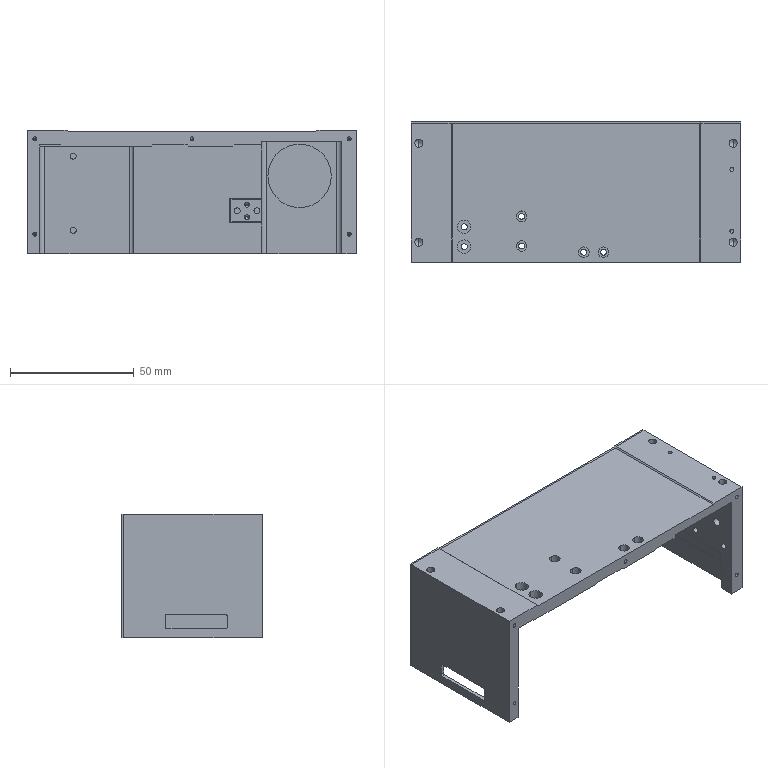NC program | NX | posted with a generic post | part box 133 x 56.74 x 50 mm
Whole program:
N10 G17 G21 G94 G90
(THREAD_MILLING , TOOL : D6.5XYD)
N12 T01 M6
N14 G54
N16 G17 G0 G90 X-43.5 Y6.5 B0. C0. S5000 M3
N18 G43 Z30. H1
N20 Z1.01
N22 G42 G94 G1 X-35.731 Y11.196 F1250. D1
N24 G2 X-34.89 Y10.873 Z1. R0.672
N26 X-34.89 Y10.873 Z0.365 I-8.61 J-4.373
N28 X-34.89 Y10.873 Z-0.27 I-8.61 J-4.373
N30 X-34.89 Y10.873 Z-0.905 I-8.61 J-4.373
N32 X-34.89 Y10.873 Z-1.54 I-8.61 J-4.373
N34 X-34.89 Y10.873 Z-2.175 I-8.61 J-4.373
N36 X-34.89 Y10.873 Z-2.81 I-8.61 J-4.373
N38 X-34.89 Y10.873 Z-3.445 I-8.61 J-4.373
N40 X-34.89 Y10.873 Z-4.08 I-8.61 J-4.373
N42 X-51.762 Y11.5 Z-4.5 R-9.657
N44 X-50.899 Y11.759 Z-4.51 R0.672
N46 G40
N48 G1 X-43.5 Y6.5
N50 G0 Z1.012
N52 G42 G1 X-35.777 Y11.271
N54 G2 X-34.819 Y10.909 Z1. R0.759
N56 X-34.819 Y10.909 Z0.365 I-8.681 J-4.409
N58 X-34.819 Y10.909 Z-0.27 I-8.681 J-4.409
N60 X-34.819 Y10.909 Z-0.905 I-8.681 J-4.409
N62 X-34.819 Y10.909 Z-1.54 I-8.681 J-4.409
N64 X-34.819 Y10.909 Z-2.175 I-8.681 J-4.409
N66 X-34.819 Y10.909 Z-2.81 I-8.681 J-4.409
N68 X-34.819 Y10.909 Z-3.445 I-8.681 J-4.409
N70 X-34.819 Y10.909 Z-4.08 I-8.681 J-4.409
N72 X-51.83 Y11.541 Z-4.5 R-9.736
N74 X-50.848 Y11.831 Z-4.512 R0.759
N76 G40
N78 G1 X-43.5 Y6.5
N80 G0 Z1.013
N82 G42 G1 X-35.824 Y11.345
N84 G2 X-34.749 Y10.945 Z1. R0.846
N86 X-34.749 Y10.945 Z0.365 I-8.751 J-4.445
N88 X-34.749 Y10.945 Z-0.27 I-8.751 J-4.445
N90 X-34.749 Y10.945 Z-0.905 I-8.751 J-4.445
N92 X-34.749 Y10.945 Z-1.54 I-8.751 J-4.445
N94 X-34.749 Y10.945 Z-2.175 I-8.751 J-4.445
N96 X-34.749 Y10.945 Z-2.81 I-8.751 J-4.445
N98 X-34.749 Y10.945 Z-3.445 I-8.751 J-4.445
N100 X-34.749 Y10.945 Z-4.08 I-8.751 J-4.445
N102 X-51.898 Y11.582 Z-4.5 R-9.816
N104 X-50.796 Y11.901 Z-4.513 R0.846
N106 G40
N108 G1 X-43.5 Y6.5
N110 G0 Z1.014
N112 G42 G1 X-35.87 Y11.418
N114 G2 X-34.678 Y10.981 Z1. R0.932
N116 X-34.678 Y10.981 Z0.365 I-8.822 J-4.481
N118 X-34.678 Y10.981 Z-0.27 I-8.822 J-4.481
N120 X-34.678 Y10.981 Z-0.905 I-8.822 J-4.481
N122 X-34.678 Y10.981 Z-1.54 I-8.822 J-4.481
N124 X-34.678 Y10.981 Z-2.175 I-8.822 J-4.481
N126 X-34.678 Y10.981 Z-2.81 I-8.822 J-4.481
N128 X-34.678 Y10.981 Z-3.445 I-8.822 J-4.481
N130 X-34.678 Y10.981 Z-4.08 I-8.822 J-4.481
N132 X-51.966 Y11.623 Z-4.5 R-9.895
N134 X-50.744 Y11.971 Z-4.514 R0.932
N136 G40
N138 G1 X-43.5 Y6.5
N140 G0 Z30.
N142 M5
N144 M2